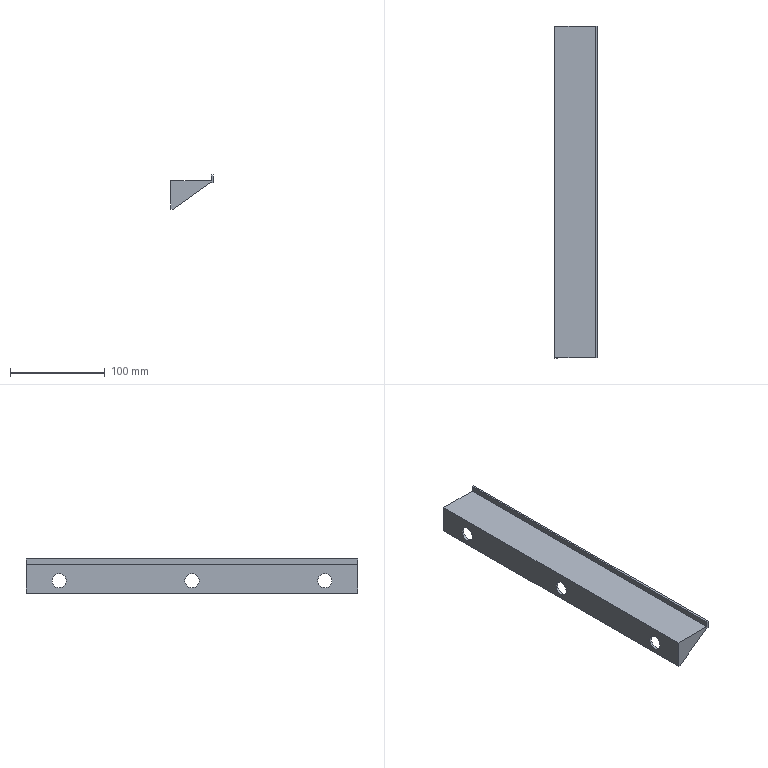Part | SolidWorks | features BaseBody 1 | 1 solid | 28 faces | box 44.5 x 350 x 36 mm | volume 59560 mm3 | plane 22 | cylinder 6 | commonest cylinder face diameters 15 x6
STEP:
#1=CARTESIAN_POINT('',(236.946,-4310.973,2209.971));
#2=VERTEX_POINT('',#1);
#3=CARTESIAN_POINT('',(236.946,-4310.973,2194.971));
#4=VERTEX_POINT('',#3);
#5=CARTESIAN_POINT('',(236.946,-4310.973,2202.471));
#6=DIRECTION('',(1.,0.,0.));
#7=DIRECTION('',(0.,0.,-1.));
#8=AXIS2_PLACEMENT_3D('',#5,#6,#7);
#9=CIRCLE('',#8,7.5);
#10=EDGE_CURVE('',#2,#4,#9,.T.);
#11=ORIENTED_EDGE('',*,*,#10,.F.);
#12=CARTESIAN_POINT('',(238.946,-4310.973,2209.971));
#13=VERTEX_POINT('',#12);
#14=CARTESIAN_POINT('',(234.817,-4310.973,2209.971));
#15=DIRECTION('',(1.,0.,0.));
#16=VECTOR('',#15,1000.);
#17=LINE('',#14,#16);
#18=EDGE_CURVE('',#2,#13,#17,.T.);
#19=ORIENTED_EDGE('',*,*,#18,.T.);
#20=CARTESIAN_POINT('',(238.946,-4310.973,2194.971));
#21=VERTEX_POINT('',#20);
#22=CARTESIAN_POINT('',(238.946,-4310.973,2202.471));
#23=DIRECTION('',(-1.,0.,0.));
#24=DIRECTION('',(0.,0.,-1.));
#25=AXIS2_PLACEMENT_3D('',#22,#23,#24);
#26=CIRCLE('',#25,7.5);
#27=EDGE_CURVE('',#21,#13,#26,.T.);
#28=ORIENTED_EDGE('',*,*,#27,.F.);
#29=CARTESIAN_POINT('',(234.817,-4310.973,2194.971));
#30=DIRECTION('',(1.,0.,0.));
#31=VECTOR('',#30,1000.);
#32=LINE('',#29,#31);
#33=EDGE_CURVE('',#4,#21,#32,.T.);
#34=ORIENTED_EDGE('',*,*,#33,.F.);
#35=EDGE_LOOP('',(#11,#19,#28,#34));
#36=FACE_OUTER_BOUND('',#35,.T.);
#37=CARTESIAN_POINT('',(234.817,-4310.973,2202.471));
#38=DIRECTION('',(1.,0.,0.));
#39=DIRECTION('',(0.,0.,-1.));
#40=AXIS2_PLACEMENT_3D('',#37,#38,#39);
#41=CYLINDRICAL_SURFACE('',#40,7.5);
#42=ADVANCED_FACE('',(#36),#41,.F.);
#43=CARTESIAN_POINT('',(238.946,-4030.973,2194.971));
#44=VERTEX_POINT('',#43);
#45=CARTESIAN_POINT('',(238.946,-4030.973,2209.971));
#46=VERTEX_POINT('',#45);
#47=CARTESIAN_POINT('',(238.946,-4030.973,2202.471));
#48=DIRECTION('',(-1.,0.,0.));
#49=DIRECTION('',(0.,0.,1.));
#50=AXIS2_PLACEMENT_3D('',#47,#48,#49);
#51=CIRCLE('',#50,7.5);
#52=EDGE_CURVE('',#44,#46,#51,.T.);
#53=ORIENTED_EDGE('',*,*,#52,.F.);
#54=CARTESIAN_POINT('',(236.946,-4030.973,2194.971));
#55=VERTEX_POINT('',#54);
#56=CARTESIAN_POINT('',(234.817,-4030.973,2194.971));
#57=DIRECTION('',(-1.,0.,0.));
#58=VECTOR('',#57,1000.);
#59=LINE('',#56,#58);
#60=EDGE_CURVE('',#44,#55,#59,.T.);
#61=ORIENTED_EDGE('',*,*,#60,.T.);
#62=CARTESIAN_POINT('',(236.946,-4030.973,2209.971));
#63=VERTEX_POINT('',#62);
#64=CARTESIAN_POINT('',(236.946,-4030.973,2202.471));
#65=DIRECTION('',(1.,0.,0.));
#66=DIRECTION('',(0.,0.,1.));
#67=AXIS2_PLACEMENT_3D('',#64,#65,#66);
#68=CIRCLE('',#67,7.5);
#69=EDGE_CURVE('',#63,#55,#68,.T.);
#70=ORIENTED_EDGE('',*,*,#69,.F.);
#71=CARTESIAN_POINT('',(234.817,-4030.973,2209.971));
#72=DIRECTION('',(-1.,0.,0.));
#73=VECTOR('',#72,1000.);
#74=LINE('',#71,#73);
#75=EDGE_CURVE('',#46,#63,#74,.T.);
#76=ORIENTED_EDGE('',*,*,#75,.F.);
#77=EDGE_LOOP('',(#53,#61,#70,#76));
#78=FACE_OUTER_BOUND('',#77,.T.);
#79=CARTESIAN_POINT('',(234.817,-4030.973,2202.471));
#80=DIRECTION('',(-1.,0.,0.));
#81=DIRECTION('',(0.,0.,1.));
#82=AXIS2_PLACEMENT_3D('',#79,#80,#81);
#83=CYLINDRICAL_SURFACE('',#82,7.5);
#84=ADVANCED_FACE('',(#78),#83,.F.);
#85=CARTESIAN_POINT('',(238.946,-4170.973,2194.971));
#86=VERTEX_POINT('',#85);
#87=CARTESIAN_POINT('',(238.946,-4170.973,2209.971));
#88=VERTEX_POINT('',#87);
#89=CARTESIAN_POINT('',(238.946,-4170.973,2202.471));
#90=DIRECTION('',(-1.,0.,0.));
#91=DIRECTION('',(0.,0.,1.));
#92=AXIS2_PLACEMENT_3D('',#89,#90,#91);
#93=CIRCLE('',#92,7.5);
#94=EDGE_CURVE('',#86,#88,#93,.T.);
#95=ORIENTED_EDGE('',*,*,#94,.F.);
#96=CARTESIAN_POINT('',(236.946,-4170.973,2194.971));
#97=VERTEX_POINT('',#96);
#98=CARTESIAN_POINT('',(234.817,-4170.973,2194.971));
#99=DIRECTION('',(-1.,0.,0.));
#100=VECTOR('',#99,1000.);
#101=LINE('',#98,#100);
#102=EDGE_CURVE('',#86,#97,#101,.T.);
#103=ORIENTED_EDGE('',*,*,#102,.T.);
#104=CARTESIAN_POINT('',(236.946,-4170.973,2209.971));
#105=VERTEX_POINT('',#104);
#106=CARTESIAN_POINT('',(236.946,-4170.973,2202.471));
#107=DIRECTION('',(1.,0.,0.));
#108=DIRECTION('',(0.,0.,1.));
#109=AXIS2_PLACEMENT_3D('',#106,#107,#108);
#110=CIRCLE('',#109,7.5);
#111=EDGE_CURVE('',#105,#97,#110,.T.);
#112=ORIENTED_EDGE('',*,*,#111,.F.);
#113=CARTESIAN_POINT('',(234.817,-4170.973,2209.971));
#114=DIRECTION('',(-1.,0.,0.));
#115=VECTOR('',#114,1000.);
#116=LINE('',#113,#115);
#117=EDGE_CURVE('',#88,#105,#116,.T.);
#118=ORIENTED_EDGE('',*,*,#117,.F.);
#119=EDGE_LOOP('',(#95,#103,#112,#118));
#120=FACE_OUTER_BOUND('',#119,.T.);
#121=CARTESIAN_POINT('',(234.817,-4170.973,2202.471));
#122=DIRECTION('',(-1.,0.,0.));
#123=DIRECTION('',(0.,0.,1.));
#124=AXIS2_PLACEMENT_3D('',#121,#122,#123);
#125=CYLINDRICAL_SURFACE('',#124,7.5);
#126=ADVANCED_FACE('',(#120),#125,.F.);
#127=CARTESIAN_POINT('',(279.446,-3995.973,2219.471));
#128=VERTEX_POINT('',#127);
#129=CARTESIAN_POINT('',(236.946,-3995.973,2219.471));
#130=VERTEX_POINT('',#129);
#131=CARTESIAN_POINT('',(277.446,-3995.973,2219.471));
#132=DIRECTION('',(-1.,0.,0.));
#133=VECTOR('',#132,1000.);
#134=LINE('',#131,#133);
#135=EDGE_CURVE('',#128,#130,#134,.T.);
#136=ORIENTED_EDGE('',*,*,#135,.T.);
#137=CARTESIAN_POINT('',(236.946,-4345.973,2219.471));
#138=VERTEX_POINT('',#137);
#139=CARTESIAN_POINT('',(236.946,-3995.973,2219.471));
#140=DIRECTION('',(0.,-1.,0.));
#141=VECTOR('',#140,1000.);
#142=LINE('',#139,#141);
#143=EDGE_CURVE('',#130,#138,#142,.T.);
#144=ORIENTED_EDGE('',*,*,#143,.T.);
#145=CARTESIAN_POINT('',(279.446,-4345.973,2219.471));
#146=VERTEX_POINT('',#145);
#147=CARTESIAN_POINT('',(277.446,-4345.973,2219.471));
#148=DIRECTION('',(1.,0.,0.));
#149=VECTOR('',#148,1000.);
#150=LINE('',#147,#149);
#151=EDGE_CURVE('',#138,#146,#150,.T.);
#152=ORIENTED_EDGE('',*,*,#151,.T.);
#153=CARTESIAN_POINT('',(279.446,-3995.973,2219.471));
#154=DIRECTION('',(0.,1.,0.));
#155=VECTOR('',#154,1000.);
#156=LINE('',#153,#155);
#157=EDGE_CURVE('',#146,#128,#156,.T.);
#158=ORIENTED_EDGE('',*,*,#157,.T.);
#159=EDGE_LOOP('',(#136,#144,#152,#158));
#160=FACE_OUTER_BOUND('',#159,.T.);
#161=CARTESIAN_POINT('',(277.446,-3995.973,2219.471));
#162=DIRECTION('',(0.,0.,1.));
#163=DIRECTION('',(1.,0.,0.));
#164=AXIS2_PLACEMENT_3D('',#161,#162,#163);
#165=PLANE('',#164);
#166=ADVANCED_FACE('',(#160),#165,.T.);
#167=CARTESIAN_POINT('',(236.946,-4345.973,2189.471));
#168=VERTEX_POINT('',#167);
#169=CARTESIAN_POINT('',(236.946,-4345.973,2189.471));
#170=DIRECTION('',(0.,0.,1.));
#171=VECTOR('',#170,1000.);
#172=LINE('',#169,#171);
#173=EDGE_CURVE('',#168,#138,#172,.T.);
#174=ORIENTED_EDGE('',*,*,#173,.T.);
#175=ORIENTED_EDGE('',*,*,#143,.F.);
#176=CARTESIAN_POINT('',(236.946,-3995.973,2189.471));
#177=VERTEX_POINT('',#176);
#178=CARTESIAN_POINT('',(236.946,-3995.973,2189.471));
#179=DIRECTION('',(0.,0.,-1.));
#180=VECTOR('',#179,1000.);
#181=LINE('',#178,#180);
#182=EDGE_CURVE('',#130,#177,#181,.T.);
#183=ORIENTED_EDGE('',*,*,#182,.T.);
#184=CARTESIAN_POINT('',(236.946,-3998.473,2189.471));
#185=DIRECTION('',(0.,-1.,0.));
#186=VECTOR('',#185,1000.);
#187=LINE('',#184,#186);
#188=EDGE_CURVE('',#177,#168,#187,.T.);
#189=ORIENTED_EDGE('',*,*,#188,.T.);
#190=EDGE_LOOP('',(#174,#175,#183,#189));
#191=FACE_OUTER_BOUND('',#190,.T.);
#192=CARTESIAN_POINT('',(236.946,-4310.973,2202.471));
#193=DIRECTION('',(1.,0.,0.));
#194=DIRECTION('',(0.,0.,-1.));
#195=AXIS2_PLACEMENT_3D('',#192,#193,#194);
#196=CIRCLE('',#195,7.5);
#197=EDGE_CURVE('',#4,#2,#196,.T.);
#198=ORIENTED_EDGE('',*,*,#197,.T.);
#199=ORIENTED_EDGE('',*,*,#10,.T.);
#200=EDGE_LOOP('',(#198,#199));
#201=FACE_BOUND('',#200,.T.);
#202=ORIENTED_EDGE('',*,*,#69,.T.);
#203=CARTESIAN_POINT('',(236.946,-4030.973,2202.471));
#204=DIRECTION('',(1.,0.,0.));
#205=DIRECTION('',(0.,0.,1.));
#206=AXIS2_PLACEMENT_3D('',#203,#204,#205);
#207=CIRCLE('',#206,7.5);
#208=EDGE_CURVE('',#55,#63,#207,.T.);
#209=ORIENTED_EDGE('',*,*,#208,.T.);
#210=EDGE_LOOP('',(#202,#209));
#211=FACE_BOUND('',#210,.T.);
#212=ORIENTED_EDGE('',*,*,#111,.T.);
#213=CARTESIAN_POINT('',(236.946,-4170.973,2202.471));
#214=DIRECTION('',(1.,0.,0.));
#215=DIRECTION('',(0.,0.,1.));
#216=AXIS2_PLACEMENT_3D('',#213,#214,#215);
#217=CIRCLE('',#216,7.5);
#218=EDGE_CURVE('',#97,#105,#217,.T.);
#219=ORIENTED_EDGE('',*,*,#218,.T.);
#220=EDGE_LOOP('',(#212,#219));
#221=FACE_BOUND('',#220,.T.);
#222=CARTESIAN_POINT('',(236.946,-3998.473,2189.471));
#223=DIRECTION('',(-1.,0.,0.));
#224=DIRECTION('',(0.,0.,1.));
#225=AXIS2_PLACEMENT_3D('',#222,#223,#224);
#226=PLANE('',#225);
#227=ADVANCED_FACE('',(#191,#201,#211,#221),#226,.T.);
#228=CARTESIAN_POINT('',(239.446,-3995.973,2189.471));
#229=VERTEX_POINT('',#228);
#230=CARTESIAN_POINT('',(253.175,-3995.973,2189.471));
#231=DIRECTION('',(1.,0.,0.));
#232=VECTOR('',#231,1000.);
#233=LINE('',#230,#232);
#234=EDGE_CURVE('',#177,#229,#233,.T.);
#235=ORIENTED_EDGE('',*,*,#234,.F.);
#236=ORIENTED_EDGE('',*,*,#182,.F.);
#237=ORIENTED_EDGE('',*,*,#135,.F.);
#238=CARTESIAN_POINT('',(279.446,-3995.973,2225.471));
#239=VERTEX_POINT('',#238);
#240=CARTESIAN_POINT('',(279.446,-3995.973,2208.045));
#241=DIRECTION('',(0.,0.,-1.));
#242=VECTOR('',#241,1000.);
#243=LINE('',#240,#242);
#244=EDGE_CURVE('',#239,#128,#243,.T.);
#245=ORIENTED_EDGE('',*,*,#244,.F.);
#246=CARTESIAN_POINT('',(281.446,-3995.973,2225.471));
#247=VERTEX_POINT('',#246);
#248=CARTESIAN_POINT('',(253.175,-3995.973,2225.471));
#249=DIRECTION('',(-1.,0.,0.));
#250=VECTOR('',#249,1000.);
#251=LINE('',#248,#250);
#252=EDGE_CURVE('',#247,#239,#251,.T.);
#253=ORIENTED_EDGE('',*,*,#252,.F.);
#254=CARTESIAN_POINT('',(281.446,-3995.973,2217.471));
#255=VERTEX_POINT('',#254);
#256=CARTESIAN_POINT('',(281.446,-3995.973,2208.045));
#257=DIRECTION('',(0.,0.,1.));
#258=VECTOR('',#257,1000.);
#259=LINE('',#256,#258);
#260=EDGE_CURVE('',#255,#247,#259,.T.);
#261=ORIENTED_EDGE('',*,*,#260,.F.);
#262=CARTESIAN_POINT('',(278.946,-3995.973,2217.471));
#263=VERTEX_POINT('',#262);
#264=CARTESIAN_POINT('',(253.175,-3995.973,2217.471));
#265=DIRECTION('',(1.,0.,0.));
#266=VECTOR('',#265,1000.);
#267=LINE('',#264,#266);
#268=EDGE_CURVE('',#263,#255,#267,.T.);
#269=ORIENTED_EDGE('',*,*,#268,.F.);
#270=CARTESIAN_POINT('',(239.446,-3995.973,2189.471));
#271=DIRECTION('',(0.8158,0.,0.5783));
#272=VECTOR('',#271,1000.);
#273=LINE('',#270,#272);
#274=EDGE_CURVE('',#229,#263,#273,.T.);
#275=ORIENTED_EDGE('',*,*,#274,.F.);
#276=EDGE_LOOP('',(#235,#236,#237,#245,#253,#261,#269,#275));
#277=FACE_OUTER_BOUND('',#276,.T.);
#278=CARTESIAN_POINT('',(253.175,-3995.973,2208.045));
#279=DIRECTION('',(0.,-1.,0.));
#280=DIRECTION('',(0.,0.,-1.));
#281=AXIS2_PLACEMENT_3D('',#278,#279,#280);
#282=PLANE('',#281);
#283=ADVANCED_FACE('',(#277),#282,.F.);
#284=ORIENTED_EDGE('',*,*,#244,.T.);
#285=ORIENTED_EDGE('',*,*,#157,.F.);
#286=CARTESIAN_POINT('',(279.446,-4345.973,2225.471));
#287=VERTEX_POINT('',#286);
#288=CARTESIAN_POINT('',(279.446,-4345.973,2225.471));
#289=DIRECTION('',(0.,0.,1.));
#290=VECTOR('',#289,1000.);
#291=LINE('',#288,#290);
#292=EDGE_CURVE('',#146,#287,#291,.T.);
#293=ORIENTED_EDGE('',*,*,#292,.T.);
#294=CARTESIAN_POINT('',(279.446,-3995.973,2225.471));
#295=DIRECTION('',(0.,1.,0.));
#296=VECTOR('',#295,1000.);
#297=LINE('',#294,#296);
#298=EDGE_CURVE('',#287,#239,#297,.T.);
#299=ORIENTED_EDGE('',*,*,#298,.T.);
#300=EDGE_LOOP('',(#284,#285,#293,#299));
#301=FACE_OUTER_BOUND('',#300,.T.);
#302=CARTESIAN_POINT('',(279.446,-3995.973,2225.471));
#303=DIRECTION('',(-1.,0.,0.));
#304=DIRECTION('',(0.,0.,1.));
#305=AXIS2_PLACEMENT_3D('',#302,#303,#304);
#306=PLANE('',#305);
#307=ADVANCED_FACE('',(#301),#306,.T.);
#308=CARTESIAN_POINT('',(278.946,-4345.973,2217.471));
#309=VERTEX_POINT('',#308);
#310=CARTESIAN_POINT('',(239.446,-4345.973,2189.471));
#311=VERTEX_POINT('',#310);
#312=CARTESIAN_POINT('',(278.946,-4345.973,2217.471));
#313=DIRECTION('',(-0.8158,0.,-0.5783));
#314=VECTOR('',#313,1000.);
#315=LINE('',#312,#314);
#316=EDGE_CURVE('',#309,#311,#315,.T.);
#317=ORIENTED_EDGE('',*,*,#316,.F.);
#318=CARTESIAN_POINT('',(281.446,-4345.973,2217.471));
#319=VERTEX_POINT('',#318);
#320=CARTESIAN_POINT('',(253.175,-4345.973,2217.471));
#321=DIRECTION('',(-1.,0.,0.));
#322=VECTOR('',#321,1000.);
#323=LINE('',#320,#322);
#324=EDGE_CURVE('',#319,#309,#323,.T.);
#325=ORIENTED_EDGE('',*,*,#324,.F.);
#326=CARTESIAN_POINT('',(281.446,-4345.973,2225.471));
#327=VERTEX_POINT('',#326);
#328=CARTESIAN_POINT('',(281.446,-4345.973,2208.045));
#329=DIRECTION('',(0.,0.,-1.));
#330=VECTOR('',#329,1000.);
#331=LINE('',#328,#330);
#332=EDGE_CURVE('',#327,#319,#331,.T.);
#333=ORIENTED_EDGE('',*,*,#332,.F.);
#334=CARTESIAN_POINT('',(253.175,-4345.973,2225.471));
#335=DIRECTION('',(1.,0.,0.));
#336=VECTOR('',#335,1000.);
#337=LINE('',#334,#336);
#338=EDGE_CURVE('',#287,#327,#337,.T.);
#339=ORIENTED_EDGE('',*,*,#338,.F.);
#340=ORIENTED_EDGE('',*,*,#292,.F.);
#341=ORIENTED_EDGE('',*,*,#151,.F.);
#342=ORIENTED_EDGE('',*,*,#173,.F.);
#343=CARTESIAN_POINT('',(253.175,-4345.973,2189.471));
#344=DIRECTION('',(-1.,0.,0.));
#345=VECTOR('',#344,1000.);
#346=LINE('',#343,#345);
#347=EDGE_CURVE('',#311,#168,#346,.T.);
#348=ORIENTED_EDGE('',*,*,#347,.F.);
#349=EDGE_LOOP('',(#317,#325,#333,#339,#340,#341,#342,#348));
#350=FACE_OUTER_BOUND('',#349,.T.);
#351=CARTESIAN_POINT('',(253.175,-4345.973,2208.045));
#352=DIRECTION('',(0.,1.,0.));
#353=DIRECTION('',(0.,0.,1.));
#354=AXIS2_PLACEMENT_3D('',#351,#352,#353);
#355=PLANE('',#354);
#356=ADVANCED_FACE('',(#350),#355,.F.);
#357=ORIENTED_EDGE('',*,*,#347,.T.);
#358=ORIENTED_EDGE('',*,*,#188,.F.);
#359=ORIENTED_EDGE('',*,*,#234,.T.);
#360=CARTESIAN_POINT('',(239.446,-3998.473,2189.471));
#361=VERTEX_POINT('',#360);
#362=CARTESIAN_POINT('',(239.446,-3998.473,2189.471));
#363=DIRECTION('',(0.,-1.,0.));
#364=VECTOR('',#363,1000.);
#365=LINE('',#362,#364);
#366=EDGE_CURVE('',#229,#361,#365,.T.);
#367=ORIENTED_EDGE('',*,*,#366,.T.);
#368=CARTESIAN_POINT('',(238.946,-3998.473,2189.471));
#369=VERTEX_POINT('',#368);
#370=CARTESIAN_POINT('',(253.175,-3998.473,2189.471));
#371=DIRECTION('',(1.,0.,0.));
#372=VECTOR('',#371,1000.);
#373=LINE('',#370,#372);
#374=EDGE_CURVE('',#369,#361,#373,.T.);
#375=ORIENTED_EDGE('',*,*,#374,.F.);
#376=CARTESIAN_POINT('',(238.946,-4095.973,2189.471));
#377=VERTEX_POINT('',#376);
#378=CARTESIAN_POINT('',(238.946,-3998.473,2189.471));
#379=DIRECTION('',(0.,-1.,0.));
#380=VECTOR('',#379,1000.);
#381=LINE('',#378,#380);
#382=EDGE_CURVE('',#369,#377,#381,.T.);
#383=ORIENTED_EDGE('',*,*,#382,.T.);
#384=CARTESIAN_POINT('',(239.446,-4095.973,2189.471));
#385=VERTEX_POINT('',#384);
#386=CARTESIAN_POINT('',(253.175,-4095.973,2189.471));
#387=DIRECTION('',(1.,0.,0.));
#388=VECTOR('',#387,1000.);
#389=LINE('',#386,#388);
#390=EDGE_CURVE('',#377,#385,#389,.T.);
#391=ORIENTED_EDGE('',*,*,#390,.T.);
#392=CARTESIAN_POINT('',(239.446,-4098.473,2189.471));
#393=VERTEX_POINT('',#392);
#394=CARTESIAN_POINT('',(239.446,-3998.473,2189.471));
#395=DIRECTION('',(0.,-1.,0.));
#396=VECTOR('',#395,1000.);
#397=LINE('',#394,#396);
#398=EDGE_CURVE('',#385,#393,#397,.T.);
#399=ORIENTED_EDGE('',*,*,#398,.T.);
#400=CARTESIAN_POINT('',(238.946,-4098.473,2189.471));
#401=VERTEX_POINT('',#400);
#402=CARTESIAN_POINT('',(253.175,-4098.473,2189.471));
#403=DIRECTION('',(1.,0.,0.));
#404=VECTOR('',#403,1000.);
#405=LINE('',#402,#404);
#406=EDGE_CURVE('',#401,#393,#405,.T.);
#407=ORIENTED_EDGE('',*,*,#406,.F.);
#408=CARTESIAN_POINT('',(238.946,-4243.473,2189.471));
#409=VERTEX_POINT('',#408);
#410=CARTESIAN_POINT('',(238.946,-3998.473,2189.471));
#411=DIRECTION('',(0.,-1.,0.));
#412=VECTOR('',#411,1000.);
#413=LINE('',#410,#412);
#414=EDGE_CURVE('',#401,#409,#413,.T.);
#415=ORIENTED_EDGE('',*,*,#414,.T.);
#416=CARTESIAN_POINT('',(239.446,-4243.473,2189.471));
#417=VERTEX_POINT('',#416);
#418=CARTESIAN_POINT('',(253.175,-4243.473,2189.471));
#419=DIRECTION('',(-1.,0.,0.));
#420=VECTOR('',#419,1000.);
#421=LINE('',#418,#420);
#422=EDGE_CURVE('',#417,#409,#421,.T.);
#423=ORIENTED_EDGE('',*,*,#422,.F.);
#424=CARTESIAN_POINT('',(239.446,-4245.973,2189.471));
#425=VERTEX_POINT('',#424);
#426=CARTESIAN_POINT('',(239.446,-3998.473,2189.471));
#427=DIRECTION('',(0.,-1.,0.));
#428=VECTOR('',#427,1000.);
#429=LINE('',#426,#428);
#430=EDGE_CURVE('',#417,#425,#429,.T.);
#431=ORIENTED_EDGE('',*,*,#430,.T.);
#432=CARTESIAN_POINT('',(238.946,-4245.973,2189.471));
#433=VERTEX_POINT('',#432);
#434=CARTESIAN_POINT('',(253.175,-4245.973,2189.471));
#435=DIRECTION('',(-1.,0.,0.));
#436=VECTOR('',#435,1000.);
#437=LINE('',#434,#436);
#438=EDGE_CURVE('',#425,#433,#437,.T.);
#439=ORIENTED_EDGE('',*,*,#438,.T.);
#440=CARTESIAN_POINT('',(238.946,-4343.473,2189.471));
#441=VERTEX_POINT('',#440);
#442=CARTESIAN_POINT('',(238.946,-3998.473,2189.471));
#443=DIRECTION('',(0.,-1.,0.));
#444=VECTOR('',#443,1000.);
#445=LINE('',#442,#444);
#446=EDGE_CURVE('',#433,#441,#445,.T.);
#447=ORIENTED_EDGE('',*,*,#446,.T.);
#448=CARTESIAN_POINT('',(239.446,-4343.473,2189.471));
#449=VERTEX_POINT('',#448);
#450=CARTESIAN_POINT('',(253.175,-4343.473,2189.471));
#451=DIRECTION('',(-1.,0.,0.));
#452=VECTOR('',#451,1000.);
#453=LINE('',#450,#452);
#454=EDGE_CURVE('',#449,#441,#453,.T.);
#455=ORIENTED_EDGE('',*,*,#454,.F.);
#456=CARTESIAN_POINT('',(239.446,-3998.473,2189.471));
#457=DIRECTION('',(0.,-1.,0.));
#458=VECTOR('',#457,1000.);
#459=LINE('',#456,#458);
#460=EDGE_CURVE('',#449,#311,#459,.T.);
#461=ORIENTED_EDGE('',*,*,#460,.T.);
#462=EDGE_LOOP('',(#357,#358,#359,#367,#375,#383,#391,#399,#407,#415,#423,#431,#439,#447,#455,#461));
#463=FACE_OUTER_BOUND('',#462,.T.);
#464=CARTESIAN_POINT('',(239.446,-3998.473,2189.471));
#465=DIRECTION('',(0.,0.,-1.));
#466=DIRECTION('',(-1.,0.,0.));
#467=AXIS2_PLACEMENT_3D('',#464,#465,#466);
#468=PLANE('',#467);
#469=ADVANCED_FACE('',(#463),#468,.T.);
#470=ORIENTED_EDGE('',*,*,#18,.F.);
#471=ORIENTED_EDGE('',*,*,#197,.F.);
#472=ORIENTED_EDGE('',*,*,#33,.T.);
#473=CARTESIAN_POINT('',(238.946,-4310.973,2202.471));
#474=DIRECTION('',(-1.,0.,0.));
#475=DIRECTION('',(0.,0.,-1.));
#476=AXIS2_PLACEMENT_3D('',#473,#474,#475);
#477=CIRCLE('',#476,7.5);
#478=EDGE_CURVE('',#13,#21,#477,.T.);
#479=ORIENTED_EDGE('',*,*,#478,.F.);
#480=EDGE_LOOP('',(#470,#471,#472,#479));
#481=FACE_OUTER_BOUND('',#480,.T.);
#482=CARTESIAN_POINT('',(234.817,-4310.973,2202.471));
#483=DIRECTION('',(1.,0.,0.));
#484=DIRECTION('',(0.,0.,-1.));
#485=AXIS2_PLACEMENT_3D('',#482,#483,#484);
#486=CYLINDRICAL_SURFACE('',#485,7.5);
#487=ADVANCED_FACE('',(#481),#486,.F.);
#488=ORIENTED_EDGE('',*,*,#60,.F.);
#489=CARTESIAN_POINT('',(238.946,-4030.973,2202.471));
#490=DIRECTION('',(-1.,0.,0.));
#491=DIRECTION('',(0.,0.,1.));
#492=AXIS2_PLACEMENT_3D('',#489,#490,#491);
#493=CIRCLE('',#492,7.5);
#494=EDGE_CURVE('',#46,#44,#493,.T.);
#495=ORIENTED_EDGE('',*,*,#494,.F.);
#496=ORIENTED_EDGE('',*,*,#75,.T.);
#497=ORIENTED_EDGE('',*,*,#208,.F.);
#498=EDGE_LOOP('',(#488,#495,#496,#497));
#499=FACE_OUTER_BOUND('',#498,.T.);
#500=CARTESIAN_POINT('',(234.817,-4030.973,2202.471));
#501=DIRECTION('',(-1.,0.,0.));
#502=DIRECTION('',(0.,0.,1.));
#503=AXIS2_PLACEMENT_3D('',#500,#501,#502);
#504=CYLINDRICAL_SURFACE('',#503,7.5);
#505=ADVANCED_FACE('',(#499),#504,.F.);
#506=ORIENTED_EDGE('',*,*,#102,.F.);
#507=CARTESIAN_POINT('',(238.946,-4170.973,2202.471));
#508=DIRECTION('',(-1.,0.,0.));
#509=DIRECTION('',(0.,0.,1.));
#510=AXIS2_PLACEMENT_3D('',#507,#508,#509);
#511=CIRCLE('',#510,7.5);
#512=EDGE_CURVE('',#88,#86,#511,.T.);
#513=ORIENTED_EDGE('',*,*,#512,.F.);
#514=ORIENTED_EDGE('',*,*,#117,.T.);
#515=ORIENTED_EDGE('',*,*,#218,.F.);
#516=EDGE_LOOP('',(#506,#513,#514,#515));
#517=FACE_OUTER_BOUND('',#516,.T.);
#518=CARTESIAN_POINT('',(234.817,-4170.973,2202.471));
#519=DIRECTION('',(-1.,0.,0.));
#520=DIRECTION('',(0.,0.,1.));
#521=AXIS2_PLACEMENT_3D('',#518,#519,#520);
#522=CYLINDRICAL_SURFACE('',#521,7.5);
#523=ADVANCED_FACE('',(#517),#522,.F.);
#524=CARTESIAN_POINT('',(278.946,-3998.473,2217.471));
#525=VERTEX_POINT('',#524);
#526=CARTESIAN_POINT('',(278.946,-3998.473,2217.471));
#527=DIRECTION('',(-0.8158,0.,-0.5783));
#528=VECTOR('',#527,1000.);
#529=LINE('',#526,#528);
#530=EDGE_CURVE('',#525,#361,#529,.T.);
#531=ORIENTED_EDGE('',*,*,#530,.T.);
#532=ORIENTED_EDGE('',*,*,#366,.F.);
#533=ORIENTED_EDGE('',*,*,#274,.T.);
#534=CARTESIAN_POINT('',(278.946,-3998.473,2217.471));
#535=DIRECTION('',(0.,-1.,0.));
#536=VECTOR('',#535,1000.);
#537=LINE('',#534,#536);
#538=EDGE_CURVE('',#263,#525,#537,.T.);
#539=ORIENTED_EDGE('',*,*,#538,.T.);
#540=EDGE_LOOP('',(#531,#532,#533,#539));
#541=FACE_OUTER_BOUND('',#540,.T.);
#542=CARTESIAN_POINT('',(278.946,-3998.473,2217.471));
#543=DIRECTION('',(0.5783,0.,-0.8158));
#544=DIRECTION('',(-0.8158,0.,-0.5783));
#545=AXIS2_PLACEMENT_3D('',#542,#543,#544);
#546=PLANE('',#545);
#547=ADVANCED_FACE('',(#541),#546,.T.);
#548=ORIENTED_EDGE('',*,*,#252,.T.);
#549=ORIENTED_EDGE('',*,*,#298,.F.);
#550=ORIENTED_EDGE('',*,*,#338,.T.);
#551=CARTESIAN_POINT('',(281.446,-3995.973,2225.471));
#552=DIRECTION('',(0.,1.,0.));
#553=VECTOR('',#552,1000.);
#554=LINE('',#551,#553);
#555=EDGE_CURVE('',#327,#247,#554,.T.);
#556=ORIENTED_EDGE('',*,*,#555,.T.);
#557=EDGE_LOOP('',(#548,#549,#550,#556));
#558=FACE_OUTER_BOUND('',#557,.T.);
#559=CARTESIAN_POINT('',(279.446,-3995.973,2225.471));
#560=DIRECTION('',(0.,0.,1.));
#561=DIRECTION('',(1.,0.,0.));
#562=AXIS2_PLACEMENT_3D('',#559,#560,#561);
#563=PLANE('',#562);
#564=ADVANCED_FACE('',(#558),#563,.T.);
#565=ORIENTED_EDGE('',*,*,#260,.T.);
#566=ORIENTED_EDGE('',*,*,#555,.F.);
#567=ORIENTED_EDGE('',*,*,#332,.T.);
#568=CARTESIAN_POINT('',(281.446,-3995.973,2217.471));
#569=DIRECTION('',(0.,1.,0.));
#570=VECTOR('',#569,1000.);
#571=LINE('',#568,#570);
#572=EDGE_CURVE('',#319,#255,#571,.T.);
#573=ORIENTED_EDGE('',*,*,#572,.T.);
#574=EDGE_LOOP('',(#565,#566,#567,#573));
#575=FACE_OUTER_BOUND('',#574,.T.);
#576=CARTESIAN_POINT('',(281.446,-3995.973,2217.471));
#577=DIRECTION('',(1.,0.,0.));
#578=DIRECTION('',(0.,0.,-1.));
#579=AXIS2_PLACEMENT_3D('',#576,#577,#578);
#580=PLANE('',#579);
#581=ADVANCED_FACE('',(#575),#580,.T.);
#582=CARTESIAN_POINT('',(238.946,-4095.973,2217.471));
#583=VERTEX_POINT('',#582);
#584=CARTESIAN_POINT('',(238.946,-3998.473,2217.471));
#585=VERTEX_POINT('',#584);
#586=CARTESIAN_POINT('',(238.946,-3995.973,2217.471));
#587=DIRECTION('',(0.,1.,0.));
#588=VECTOR('',#587,1000.);
#589=LINE('',#586,#588);
#590=EDGE_CURVE('',#583,#585,#589,.T.);
#591=ORIENTED_EDGE('',*,*,#590,.T.);
#592=CARTESIAN_POINT('',(271.446,-3998.473,2217.471));
#593=DIRECTION('',(1.,0.,0.));
#594=VECTOR('',#593,1000.);
#595=LINE('',#592,#594);
#596=EDGE_CURVE('',#585,#525,#595,.T.);
#597=ORIENTED_EDGE('',*,*,#596,.T.);
#598=ORIENTED_EDGE('',*,*,#538,.F.);
#599=ORIENTED_EDGE('',*,*,#268,.T.);
#600=ORIENTED_EDGE('',*,*,#572,.F.);
#601=ORIENTED_EDGE('',*,*,#324,.T.);
#602=CARTESIAN_POINT('',(278.946,-4343.473,2217.471));
#603=VERTEX_POINT('',#602);
#604=CARTESIAN_POINT('',(278.946,-3995.973,2217.471));
#605=DIRECTION('',(0.,1.,0.));
#606=VECTOR('',#605,1000.);
#607=LINE('',#604,#606);
#608=EDGE_CURVE('',#309,#603,#607,.T.);
#609=ORIENTED_EDGE('',*,*,#608,.T.);
#610=CARTESIAN_POINT('',(238.946,-4343.473,2217.471));
#611=VERTEX_POINT('',#610);
#612=CARTESIAN_POINT('',(271.446,-4343.473,2217.471));
#613=DIRECTION('',(-1.,0.,0.));
#614=VECTOR('',#613,1000.);
#615=LINE('',#612,#614);
#616=EDGE_CURVE('',#603,#611,#615,.T.);
#617=ORIENTED_EDGE('',*,*,#616,.T.);
#618=CARTESIAN_POINT('',(238.946,-4245.973,2217.471));
#619=VERTEX_POINT('',#618);
#620=CARTESIAN_POINT('',(238.946,-3995.973,2217.471));
#621=DIRECTION('',(0.,1.,0.));
#622=VECTOR('',#621,1000.);
#623=LINE('',#620,#622);
#624=EDGE_CURVE('',#611,#619,#623,.T.);
#625=ORIENTED_EDGE('',*,*,#624,.T.);
#626=CARTESIAN_POINT('',(278.946,-4245.973,2217.471));
#627=VERTEX_POINT('',#626);
#628=CARTESIAN_POINT('',(271.446,-4245.973,2217.471));
#629=DIRECTION('',(1.,0.,0.));
#630=VECTOR('',#629,1000.);
#631=LINE('',#628,#630);
#632=EDGE_CURVE('',#619,#627,#631,.T.);
#633=ORIENTED_EDGE('',*,*,#632,.T.);
#634=CARTESIAN_POINT('',(278.946,-4243.473,2217.471));
#635=VERTEX_POINT('',#634);
#636=CARTESIAN_POINT('',(278.946,-3995.973,2217.471));
#637=DIRECTION('',(0.,1.,0.));
#638=VECTOR('',#637,1000.);
#639=LINE('',#636,#638);
#640=EDGE_CURVE('',#627,#635,#639,.T.);
#641=ORIENTED_EDGE('',*,*,#640,.T.);
#642=CARTESIAN_POINT('',(238.946,-4243.473,2217.471));
#643=VERTEX_POINT('',#642);
#644=CARTESIAN_POINT('',(271.446,-4243.473,2217.471));
#645=DIRECTION('',(-1.,0.,0.));
#646=VECTOR('',#645,1000.);
#647=LINE('',#644,#646);
#648=EDGE_CURVE('',#635,#643,#647,.T.);
#649=ORIENTED_EDGE('',*,*,#648,.T.);
#650=CARTESIAN_POINT('',(238.946,-4098.473,2217.471));
#651=VERTEX_POINT('',#650);
#652=CARTESIAN_POINT('',(238.946,-3995.973,2217.471));
#653=DIRECTION('',(0.,1.,0.));
#654=VECTOR('',#653,1000.);
#655=LINE('',#652,#654);
#656=EDGE_CURVE('',#643,#651,#655,.T.);
#657=ORIENTED_EDGE('',*,*,#656,.T.);
#658=CARTESIAN_POINT('',(278.946,-4098.473,2217.471));
#659=VERTEX_POINT('',#658);
#660=CARTESIAN_POINT('',(271.446,-4098.473,2217.471));
#661=DIRECTION('',(1.,0.,0.));
#662=VECTOR('',#661,1000.);
#663=LINE('',#660,#662);
#664=EDGE_CURVE('',#651,#659,#663,.T.);
#665=ORIENTED_EDGE('',*,*,#664,.T.);
#666=CARTESIAN_POINT('',(278.946,-4095.973,2217.471));
#667=VERTEX_POINT('',#666);
#668=CARTESIAN_POINT('',(278.946,-3995.973,2217.471));
#669=DIRECTION('',(0.,1.,0.));
#670=VECTOR('',#669,1000.);
#671=LINE('',#668,#670);
#672=EDGE_CURVE('',#659,#667,#671,.T.);
#673=ORIENTED_EDGE('',*,*,#672,.T.);
#674=CARTESIAN_POINT('',(271.446,-4095.973,2217.471));
#675=DIRECTION('',(-1.,0.,0.));
#676=VECTOR('',#675,1000.);
#677=LINE('',#674,#676);
#678=EDGE_CURVE('',#667,#583,#677,.T.);
#679=ORIENTED_EDGE('',*,*,#678,.T.);
#680=EDGE_LOOP('',(#591,#597,#598,#599,#600,#601,#609,#617,#625,#633,#641,#649,#657,#665,#673,#679));
#681=FACE_OUTER_BOUND('',#680,.T.);
#682=CARTESIAN_POINT('',(271.446,-3995.973,2217.471));
#683=DIRECTION('',(0.,0.,-1.));
#684=DIRECTION('',(-1.,0.,0.));
#685=AXIS2_PLACEMENT_3D('',#682,#683,#684);
#686=PLANE('',#685);
#687=ADVANCED_FACE('',(#681),#686,.T.);
#688=CARTESIAN_POINT('',(278.946,-4343.473,2217.471));
#689=DIRECTION('',(0.8158,0.,0.5783));
#690=VECTOR('',#689,1000.);
#691=LINE('',#688,#690);
#692=EDGE_CURVE('',#449,#603,#691,.T.);
#693=ORIENTED_EDGE('',*,*,#692,.T.);
#694=ORIENTED_EDGE('',*,*,#608,.F.);
#695=ORIENTED_EDGE('',*,*,#316,.T.);
#696=ORIENTED_EDGE('',*,*,#460,.F.);
#697=EDGE_LOOP('',(#693,#694,#695,#696));
#698=FACE_OUTER_BOUND('',#697,.T.);
#699=CARTESIAN_POINT('',(278.946,-4343.473,2217.471));
#700=DIRECTION('',(0.5783,0.,-0.8158));
#701=DIRECTION('',(-0.8158,0.,-0.5783));
#702=AXIS2_PLACEMENT_3D('',#699,#700,#701);
#703=PLANE('',#702);
#704=ADVANCED_FACE('',(#698),#703,.T.);
#705=ORIENTED_EDGE('',*,*,#27,.T.);
#706=ORIENTED_EDGE('',*,*,#478,.T.);
#707=EDGE_LOOP('',(#705,#706));
#708=FACE_BOUND('',#707,.T.);
#709=CARTESIAN_POINT('',(238.946,-4245.973,2199.471));
#710=DIRECTION('',(0.,0.,1.));
#711=VECTOR('',#710,1000.);
#712=LINE('',#709,#711);
#713=EDGE_CURVE('',#433,#619,#712,.T.);
#714=ORIENTED_EDGE('',*,*,#713,.T.);
#715=ORIENTED_EDGE('',*,*,#624,.F.);
#716=CARTESIAN_POINT('',(238.946,-4343.473,2199.471));
#717=DIRECTION('',(0.,0.,-1.));
#718=VECTOR('',#717,1000.);
#719=LINE('',#716,#718);
#720=EDGE_CURVE('',#611,#441,#719,.T.);
#721=ORIENTED_EDGE('',*,*,#720,.T.);
#722=ORIENTED_EDGE('',*,*,#446,.F.);
#723=EDGE_LOOP('',(#714,#715,#721,#722));
#724=FACE_OUTER_BOUND('',#723,.T.);
#725=CARTESIAN_POINT('',(238.946,-3995.973,2199.471));
#726=DIRECTION('',(1.,0.,0.));
#727=DIRECTION('',(0.,0.,-1.));
#728=AXIS2_PLACEMENT_3D('',#725,#726,#727);
#729=PLANE('',#728);
#730=ADVANCED_FACE('',(#708,#724),#729,.T.);
#731=CARTESIAN_POINT('',(278.946,-4243.473,2217.471));
#732=DIRECTION('',(0.8158,0.,0.5783));
#733=VECTOR('',#732,1000.);
#734=LINE('',#731,#733);
#735=EDGE_CURVE('',#417,#635,#734,.T.);
#736=ORIENTED_EDGE('',*,*,#735,.T.);
#737=ORIENTED_EDGE('',*,*,#640,.F.);
#738=CARTESIAN_POINT('',(278.946,-4245.973,2217.471));
#739=DIRECTION('',(-0.8158,0.,-0.5783));
#740=VECTOR('',#739,1000.);
#741=LINE('',#738,#740);
#742=EDGE_CURVE('',#627,#425,#741,.T.);
#743=ORIENTED_EDGE('',*,*,#742,.T.);
#744=ORIENTED_EDGE('',*,*,#430,.F.);
#745=EDGE_LOOP('',(#736,#737,#743,#744));
#746=FACE_OUTER_BOUND('',#745,.T.);
#747=CARTESIAN_POINT('',(278.946,-4243.473,2217.471));
#748=DIRECTION('',(0.5783,0.,-0.8158));
#749=DIRECTION('',(-0.8158,0.,-0.5783));
#750=AXIS2_PLACEMENT_3D('',#747,#748,#749);
#751=PLANE('',#750);
#752=ADVANCED_FACE('',(#746),#751,.T.);
#753=CARTESIAN_POINT('',(238.946,-4098.473,2199.471));
#754=DIRECTION('',(0.,0.,1.));
#755=VECTOR('',#754,1000.);
#756=LINE('',#753,#755);
#757=EDGE_CURVE('',#401,#651,#756,.T.);
#758=ORIENTED_EDGE('',*,*,#757,.T.);
#759=ORIENTED_EDGE('',*,*,#656,.F.);
#760=CARTESIAN_POINT('',(238.946,-4243.473,2199.471));
#761=DIRECTION('',(0.,0.,-1.));
#762=VECTOR('',#761,1000.);
#763=LINE('',#760,#762);
#764=EDGE_CURVE('',#643,#409,#763,.T.);
#765=ORIENTED_EDGE('',*,*,#764,.T.);
#766=ORIENTED_EDGE('',*,*,#414,.F.);
#767=EDGE_LOOP('',(#758,#759,#765,#766));
#768=FACE_OUTER_BOUND('',#767,.T.);
#769=ORIENTED_EDGE('',*,*,#512,.T.);
#770=ORIENTED_EDGE('',*,*,#94,.T.);
#771=EDGE_LOOP('',(#769,#770));
#772=FACE_BOUND('',#771,.T.);
#773=CARTESIAN_POINT('',(238.946,-3995.973,2199.471));
#774=DIRECTION('',(1.,0.,0.));
#775=DIRECTION('',(0.,0.,-1.));
#776=AXIS2_PLACEMENT_3D('',#773,#774,#775);
#777=PLANE('',#776);
#778=ADVANCED_FACE('',(#768,#772),#777,.T.);
#779=CARTESIAN_POINT('',(278.946,-4098.473,2217.471));
#780=DIRECTION('',(-0.8158,0.,-0.5783));
#781=VECTOR('',#780,1000.);
#782=LINE('',#779,#781);
#783=EDGE_CURVE('',#659,#393,#782,.T.);
#784=ORIENTED_EDGE('',*,*,#783,.T.);
#785=ORIENTED_EDGE('',*,*,#398,.F.);
#786=CARTESIAN_POINT('',(278.946,-4095.973,2217.471));
#787=DIRECTION('',(0.8158,0.,0.5783));
#788=VECTOR('',#787,1000.);
#789=LINE('',#786,#788);
#790=EDGE_CURVE('',#385,#667,#789,.T.);
#791=ORIENTED_EDGE('',*,*,#790,.T.);
#792=ORIENTED_EDGE('',*,*,#672,.F.);
#793=EDGE_LOOP('',(#784,#785,#791,#792));
#794=FACE_OUTER_BOUND('',#793,.T.);
#795=CARTESIAN_POINT('',(278.946,-4098.473,2217.471));
#796=DIRECTION('',(0.5783,0.,-0.8158));
#797=DIRECTION('',(-0.8158,0.,-0.5783));
#798=AXIS2_PLACEMENT_3D('',#795,#796,#797);
#799=PLANE('',#798);
#800=ADVANCED_FACE('',(#794),#799,.T.);
#801=CARTESIAN_POINT('',(238.946,-4095.973,2199.471));
#802=DIRECTION('',(0.,0.,-1.));
#803=VECTOR('',#802,1000.);
#804=LINE('',#801,#803);
#805=EDGE_CURVE('',#583,#377,#804,.T.);
#806=ORIENTED_EDGE('',*,*,#805,.T.);
#807=ORIENTED_EDGE('',*,*,#382,.F.);
#808=CARTESIAN_POINT('',(238.946,-3998.473,2199.471));
#809=DIRECTION('',(0.,0.,1.));
#810=VECTOR('',#809,1000.);
#811=LINE('',#808,#810);
#812=EDGE_CURVE('',#369,#585,#811,.T.);
#813=ORIENTED_EDGE('',*,*,#812,.T.);
#814=ORIENTED_EDGE('',*,*,#590,.F.);
#815=EDGE_LOOP('',(#806,#807,#813,#814));
#816=FACE_OUTER_BOUND('',#815,.T.);
#817=ORIENTED_EDGE('',*,*,#494,.T.);
#818=ORIENTED_EDGE('',*,*,#52,.T.);
#819=EDGE_LOOP('',(#817,#818));
#820=FACE_BOUND('',#819,.T.);
#821=CARTESIAN_POINT('',(238.946,-3995.973,2199.471));
#822=DIRECTION('',(1.,0.,0.));
#823=DIRECTION('',(0.,0.,-1.));
#824=AXIS2_PLACEMENT_3D('',#821,#822,#823);
#825=PLANE('',#824);
#826=ADVANCED_FACE('',(#816,#820),#825,.T.);
#827=ORIENTED_EDGE('',*,*,#530,.F.);
#828=ORIENTED_EDGE('',*,*,#596,.F.);
#829=ORIENTED_EDGE('',*,*,#812,.F.);
#830=ORIENTED_EDGE('',*,*,#374,.T.);
#831=EDGE_LOOP('',(#827,#828,#829,#830));
#832=FACE_OUTER_BOUND('',#831,.T.);
#833=CARTESIAN_POINT('',(253.175,-3998.473,2208.045));
#834=DIRECTION('',(0.,-1.,0.));
#835=DIRECTION('',(0.,0.,-1.));
#836=AXIS2_PLACEMENT_3D('',#833,#834,#835);
#837=PLANE('',#836);
#838=ADVANCED_FACE('',(#832),#837,.T.);
#839=ORIENTED_EDGE('',*,*,#678,.F.);
#840=ORIENTED_EDGE('',*,*,#790,.F.);
#841=ORIENTED_EDGE('',*,*,#390,.F.);
#842=ORIENTED_EDGE('',*,*,#805,.F.);
#843=EDGE_LOOP('',(#839,#840,#841,#842));
#844=FACE_OUTER_BOUND('',#843,.T.);
#845=CARTESIAN_POINT('',(253.175,-4095.973,2208.045));
#846=DIRECTION('',(0.,-1.,0.));
#847=DIRECTION('',(0.,0.,-1.));
#848=AXIS2_PLACEMENT_3D('',#845,#846,#847);
#849=PLANE('',#848);
#850=ADVANCED_FACE('',(#844),#849,.F.);
#851=ORIENTED_EDGE('',*,*,#783,.F.);
#852=ORIENTED_EDGE('',*,*,#664,.F.);
#853=ORIENTED_EDGE('',*,*,#757,.F.);
#854=ORIENTED_EDGE('',*,*,#406,.T.);
#855=EDGE_LOOP('',(#851,#852,#853,#854));
#856=FACE_OUTER_BOUND('',#855,.T.);
#857=CARTESIAN_POINT('',(253.175,-4098.473,2208.045));
#858=DIRECTION('',(0.,-1.,0.));
#859=DIRECTION('',(0.,0.,-1.));
#860=AXIS2_PLACEMENT_3D('',#857,#858,#859);
#861=PLANE('',#860);
#862=ADVANCED_FACE('',(#856),#861,.T.);
#863=ORIENTED_EDGE('',*,*,#735,.F.);
#864=ORIENTED_EDGE('',*,*,#422,.T.);
#865=ORIENTED_EDGE('',*,*,#764,.F.);
#866=ORIENTED_EDGE('',*,*,#648,.F.);
#867=EDGE_LOOP('',(#863,#864,#865,#866));
#868=FACE_OUTER_BOUND('',#867,.T.);
#869=CARTESIAN_POINT('',(253.175,-4243.473,2208.045));
#870=DIRECTION('',(0.,1.,0.));
#871=DIRECTION('',(0.,0.,1.));
#872=AXIS2_PLACEMENT_3D('',#869,#870,#871);
#873=PLANE('',#872);
#874=ADVANCED_FACE('',(#868),#873,.T.);
#875=ORIENTED_EDGE('',*,*,#438,.F.);
#876=ORIENTED_EDGE('',*,*,#742,.F.);
#877=ORIENTED_EDGE('',*,*,#632,.F.);
#878=ORIENTED_EDGE('',*,*,#713,.F.);
#879=EDGE_LOOP('',(#875,#876,#877,#878));
#880=FACE_OUTER_BOUND('',#879,.T.);
#881=CARTESIAN_POINT('',(253.175,-4245.973,2208.045));
#882=DIRECTION('',(0.,1.,0.));
#883=DIRECTION('',(0.,0.,1.));
#884=AXIS2_PLACEMENT_3D('',#881,#882,#883);
#885=PLANE('',#884);
#886=ADVANCED_FACE('',(#880),#885,.F.);
#887=ORIENTED_EDGE('',*,*,#692,.F.);
#888=ORIENTED_EDGE('',*,*,#454,.T.);
#889=ORIENTED_EDGE('',*,*,#720,.F.);
#890=ORIENTED_EDGE('',*,*,#616,.F.);
#891=EDGE_LOOP('',(#887,#888,#889,#890));
#892=FACE_OUTER_BOUND('',#891,.T.);
#893=CARTESIAN_POINT('',(253.175,-4343.473,2208.045));
#894=DIRECTION('',(0.,1.,0.));
#895=DIRECTION('',(0.,0.,1.));
#896=AXIS2_PLACEMENT_3D('',#893,#894,#895);
#897=PLANE('',#896);
#898=ADVANCED_FACE('',(#892),#897,.T.);
#899=CLOSED_SHELL('',(#42,#84,#126,#166,#227,#283,#307,#356,#469,#487,#505,#523,#547,#564,#581,#687,#704,#730,#752,#778,#800,#826,#838,#850,#862,#874,#886,#898));
#900=MANIFOLD_SOLID_BREP('',#899);
#901=CARTESIAN_POINT('',(0.,0.,0.));
#902=DIRECTION('',(0.,0.,1.));
#903=DIRECTION('',(1.,0.,0.));
#904=AXIS2_PLACEMENT_3D('',#901,#902,#903);
#905=(LENGTH_UNIT()NAMED_UNIT(*)SI_UNIT(.MILLI.,.METRE.));
#906=UNCERTAINTY_MEASURE_WITH_UNIT(LENGTH_MEASURE(0.00001),#905,'','');
#907=(NAMED_UNIT(*)PLANE_ANGLE_UNIT()SI_UNIT($,.RADIAN.));
#908=(NAMED_UNIT(*)SI_UNIT($,.STERADIAN.)SOLID_ANGLE_UNIT());
#909=(GEOMETRIC_REPRESENTATION_CONTEXT(3)GLOBAL_UNCERTAINTY_ASSIGNED_CONTEXT((#906))GLOBAL_UNIT_ASSIGNED_CONTEXT((#905,#907,#908))REPRESENTATION_CONTEXT('',''));
#910=ADVANCED_BREP_SHAPE_REPRESENTATION('',(#900,#904),#909);